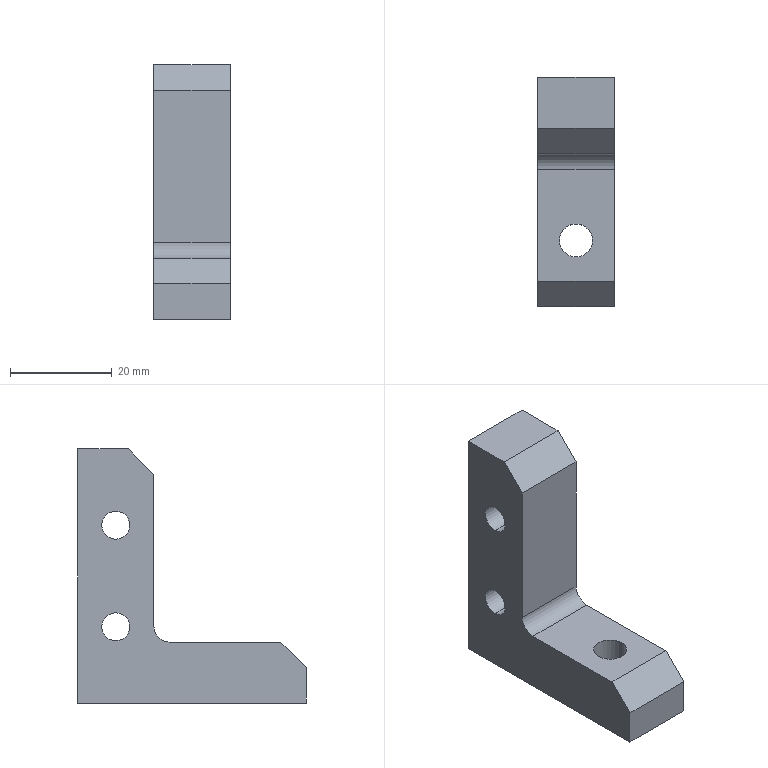Part | SolidWorks | features HoleWzd 2, Chamfer 1, Extrusion 1, Fillet 1, ICE 1 | 1 solid | 17 faces | box 15 x 45 x 50 mm | volume 15193 mm3 | plane 10 | cylinder 7 | commonest cylinder face diameters 5.5 x4 6.5 x2 6 x1
STEP:
#1=CARTESIAN_POINT('',(-7.5,0.,-7.25));
#2=VERTEX_POINT('',#1);
#3=CARTESIAN_POINT('',(-7.5,0.,-12.75));
#4=VERTEX_POINT('',#3);
#5=CARTESIAN_POINT('',(-7.5,0.,-10.));
#6=DIRECTION('',(1.,0.,0.));
#7=DIRECTION('',(0.,0.,-1.));
#8=AXIS2_PLACEMENT_3D('',#5,#6,#7);
#9=CIRCLE('',#8,2.75);
#10=EDGE_CURVE('',#2,#4,#9,.T.);
#11=ORIENTED_EDGE('',*,*,#10,.F.);
#12=CARTESIAN_POINT('',(7.5,0.,-7.25));
#13=VERTEX_POINT('',#12);
#14=CARTESIAN_POINT('',(7.5,0.,-7.25));
#15=DIRECTION('',(1.,0.,0.));
#16=VECTOR('',#15,1000.);
#17=LINE('',#14,#16);
#18=EDGE_CURVE('',#2,#13,#17,.T.);
#19=ORIENTED_EDGE('',*,*,#18,.T.);
#20=CARTESIAN_POINT('',(7.5,0.,-12.75));
#21=VERTEX_POINT('',#20);
#22=CARTESIAN_POINT('',(7.5,0.,-10.));
#23=DIRECTION('',(1.,0.,0.));
#24=DIRECTION('',(0.,0.,-1.));
#25=AXIS2_PLACEMENT_3D('',#22,#23,#24);
#26=CIRCLE('',#25,2.75);
#27=EDGE_CURVE('',#13,#21,#26,.T.);
#28=ORIENTED_EDGE('',*,*,#27,.T.);
#29=CARTESIAN_POINT('',(7.5,0.,-12.75));
#30=DIRECTION('',(1.,0.,0.));
#31=VECTOR('',#30,1000.);
#32=LINE('',#29,#31);
#33=EDGE_CURVE('',#4,#21,#32,.T.);
#34=ORIENTED_EDGE('',*,*,#33,.F.);
#35=EDGE_LOOP('',(#11,#19,#28,#34));
#36=FACE_OUTER_BOUND('',#35,.T.);
#37=CARTESIAN_POINT('',(7.5,0.,-10.));
#38=DIRECTION('',(1.,0.,0.));
#39=DIRECTION('',(0.,0.,-1.));
#40=AXIS2_PLACEMENT_3D('',#37,#38,#39);
#41=CYLINDRICAL_SURFACE('',#40,2.75);
#42=ADVANCED_FACE('',(#36),#41,.F.);
#43=CARTESIAN_POINT('',(-7.5,0.,12.75));
#44=VERTEX_POINT('',#43);
#45=CARTESIAN_POINT('',(-7.5,0.,7.25));
#46=VERTEX_POINT('',#45);
#47=CARTESIAN_POINT('',(-7.5,0.,10.));
#48=DIRECTION('',(1.,0.,0.));
#49=DIRECTION('',(0.,0.,-1.));
#50=AXIS2_PLACEMENT_3D('',#47,#48,#49);
#51=CIRCLE('',#50,2.75);
#52=EDGE_CURVE('',#44,#46,#51,.T.);
#53=ORIENTED_EDGE('',*,*,#52,.F.);
#54=CARTESIAN_POINT('',(7.5,0.,12.75));
#55=VERTEX_POINT('',#54);
#56=CARTESIAN_POINT('',(7.5,0.,12.75));
#57=DIRECTION('',(1.,0.,0.));
#58=VECTOR('',#57,1000.);
#59=LINE('',#56,#58);
#60=EDGE_CURVE('',#44,#55,#59,.T.);
#61=ORIENTED_EDGE('',*,*,#60,.T.);
#62=CARTESIAN_POINT('',(7.5,0.,7.25));
#63=VERTEX_POINT('',#62);
#64=CARTESIAN_POINT('',(7.5,0.,10.));
#65=DIRECTION('',(1.,0.,0.));
#66=DIRECTION('',(0.,0.,-1.));
#67=AXIS2_PLACEMENT_3D('',#64,#65,#66);
#68=CIRCLE('',#67,2.75);
#69=EDGE_CURVE('',#55,#63,#68,.T.);
#70=ORIENTED_EDGE('',*,*,#69,.T.);
#71=CARTESIAN_POINT('',(7.5,0.,7.25));
#72=DIRECTION('',(1.,0.,0.));
#73=VECTOR('',#72,1000.);
#74=LINE('',#71,#73);
#75=EDGE_CURVE('',#46,#63,#74,.T.);
#76=ORIENTED_EDGE('',*,*,#75,.F.);
#77=EDGE_LOOP('',(#53,#61,#70,#76));
#78=FACE_OUTER_BOUND('',#77,.T.);
#79=CARTESIAN_POINT('',(7.5,0.,10.));
#80=DIRECTION('',(1.,0.,0.));
#81=DIRECTION('',(0.,0.,-1.));
#82=AXIS2_PLACEMENT_3D('',#79,#80,#81);
#83=CYLINDRICAL_SURFACE('',#82,2.75);
#84=ADVANCED_FACE('',(#78),#83,.F.);
#85=CARTESIAN_POINT('',(-3.25,-24.5,-25.));
#86=VERTEX_POINT('',#85);
#87=CARTESIAN_POINT('',(3.25,-24.5,-25.));
#88=VERTEX_POINT('',#87);
#89=CARTESIAN_POINT('',(0.,-24.5,-25.));
#90=DIRECTION('',(0.,0.,1.));
#91=DIRECTION('',(1.,0.,0.));
#92=AXIS2_PLACEMENT_3D('',#89,#90,#91);
#93=CIRCLE('',#92,3.25);
#94=EDGE_CURVE('',#86,#88,#93,.T.);
#95=ORIENTED_EDGE('',*,*,#94,.F.);
#96=CARTESIAN_POINT('',(-3.25,-24.5,-13.));
#97=VERTEX_POINT('',#96);
#98=CARTESIAN_POINT('',(-3.25,-24.5,-13.));
#99=DIRECTION('',(0.,0.,1.));
#100=VECTOR('',#99,1000.);
#101=LINE('',#98,#100);
#102=EDGE_CURVE('',#86,#97,#101,.T.);
#103=ORIENTED_EDGE('',*,*,#102,.T.);
#104=CARTESIAN_POINT('',(3.25,-24.5,-13.));
#105=VERTEX_POINT('',#104);
#106=CARTESIAN_POINT('',(0.,-24.5,-13.));
#107=DIRECTION('',(0.,0.,1.));
#108=DIRECTION('',(1.,0.,0.));
#109=AXIS2_PLACEMENT_3D('',#106,#107,#108);
#110=CIRCLE('',#109,3.25);
#111=EDGE_CURVE('',#97,#105,#110,.T.);
#112=ORIENTED_EDGE('',*,*,#111,.T.);
#113=CARTESIAN_POINT('',(3.25,-24.5,-13.));
#114=DIRECTION('',(0.,0.,1.));
#115=VECTOR('',#114,1000.);
#116=LINE('',#113,#115);
#117=EDGE_CURVE('',#88,#105,#116,.T.);
#118=ORIENTED_EDGE('',*,*,#117,.F.);
#119=EDGE_LOOP('',(#95,#103,#112,#118));
#120=FACE_OUTER_BOUND('',#119,.T.);
#121=CARTESIAN_POINT('',(0.,-24.5,-13.));
#122=DIRECTION('',(0.,0.,1.));
#123=DIRECTION('',(1.,0.,0.));
#124=AXIS2_PLACEMENT_3D('',#121,#122,#123);
#125=CYLINDRICAL_SURFACE('',#124,3.25);
#126=ADVANCED_FACE('',(#120),#125,.F.);
#127=CARTESIAN_POINT('',(7.5,0.,-10.));
#128=DIRECTION('',(1.,0.,0.));
#129=DIRECTION('',(0.,0.,-1.));
#130=AXIS2_PLACEMENT_3D('',#127,#128,#129);
#131=CIRCLE('',#130,2.75);
#132=EDGE_CURVE('',#21,#13,#131,.T.);
#133=ORIENTED_EDGE('',*,*,#132,.F.);
#134=ORIENTED_EDGE('',*,*,#27,.F.);
#135=EDGE_LOOP('',(#133,#134));
#136=FACE_BOUND('',#135,.T.);
#137=CARTESIAN_POINT('',(7.5,0.,10.));
#138=DIRECTION('',(1.,0.,0.));
#139=DIRECTION('',(0.,0.,-1.));
#140=AXIS2_PLACEMENT_3D('',#137,#138,#139);
#141=CIRCLE('',#140,2.75);
#142=EDGE_CURVE('',#63,#55,#141,.T.);
#143=ORIENTED_EDGE('',*,*,#142,.F.);
#144=ORIENTED_EDGE('',*,*,#69,.F.);
#145=EDGE_LOOP('',(#143,#144));
#146=FACE_BOUND('',#145,.T.);
#147=CARTESIAN_POINT('',(7.5,-2.5,25.));
#148=VERTEX_POINT('',#147);
#149=CARTESIAN_POINT('',(7.5,7.5,25.));
#150=VERTEX_POINT('',#149);
#151=CARTESIAN_POINT('',(7.5,-7.5,25.));
#152=DIRECTION('',(0.,1.,0.));
#153=VECTOR('',#152,1000.);
#154=LINE('',#151,#153);
#155=EDGE_CURVE('',#148,#150,#154,.T.);
#156=ORIENTED_EDGE('',*,*,#155,.F.);
#157=CARTESIAN_POINT('',(7.5,-7.5,20.));
#158=VERTEX_POINT('',#157);
#159=CARTESIAN_POINT('',(7.5,-2.5,25.));
#160=DIRECTION('',(0.,-0.7071,-0.7071));
#161=VECTOR('',#160,1000.);
#162=LINE('',#159,#161);
#163=EDGE_CURVE('',#148,#158,#162,.T.);
#164=ORIENTED_EDGE('',*,*,#163,.T.);
#165=CARTESIAN_POINT('',(7.5,-7.5,-10.));
#166=VERTEX_POINT('',#165);
#167=CARTESIAN_POINT('',(7.5,-7.5,25.));
#168=DIRECTION('',(0.,0.,-1.));
#169=VECTOR('',#168,1000.);
#170=LINE('',#167,#169);
#171=EDGE_CURVE('',#158,#166,#170,.T.);
#172=ORIENTED_EDGE('',*,*,#171,.T.);
#173=CARTESIAN_POINT('',(7.5,-10.5,-13.));
#174=VERTEX_POINT('',#173);
#175=CARTESIAN_POINT('',(7.5,-10.5,-10.));
#176=DIRECTION('',(-1.,0.,0.));
#177=DIRECTION('',(0.,0.,1.));
#178=AXIS2_PLACEMENT_3D('',#175,#176,#177);
#179=CIRCLE('',#178,3.);
#180=EDGE_CURVE('',#166,#174,#179,.T.);
#181=ORIENTED_EDGE('',*,*,#180,.T.);
#182=CARTESIAN_POINT('',(7.5,-32.5,-13.));
#183=VERTEX_POINT('',#182);
#184=CARTESIAN_POINT('',(7.5,-7.5,-13.));
#185=DIRECTION('',(0.,-1.,0.));
#186=VECTOR('',#185,1000.);
#187=LINE('',#184,#186);
#188=EDGE_CURVE('',#174,#183,#187,.T.);
#189=ORIENTED_EDGE('',*,*,#188,.T.);
#190=CARTESIAN_POINT('',(7.5,-37.5,-18.));
#191=VERTEX_POINT('',#190);
#192=CARTESIAN_POINT('',(7.5,-37.5,-18.));
#193=DIRECTION('',(0.,-0.7071,-0.7071));
#194=VECTOR('',#193,1000.);
#195=LINE('',#192,#194);
#196=EDGE_CURVE('',#183,#191,#195,.T.);
#197=ORIENTED_EDGE('',*,*,#196,.T.);
#198=CARTESIAN_POINT('',(7.5,-37.5,-25.));
#199=VERTEX_POINT('',#198);
#200=CARTESIAN_POINT('',(7.5,-37.5,-13.));
#201=DIRECTION('',(0.,0.,-1.));
#202=VECTOR('',#201,1000.);
#203=LINE('',#200,#202);
#204=EDGE_CURVE('',#191,#199,#203,.T.);
#205=ORIENTED_EDGE('',*,*,#204,.T.);
#206=CARTESIAN_POINT('',(7.5,7.5,-25.));
#207=VERTEX_POINT('',#206);
#208=CARTESIAN_POINT('',(7.5,-7.5,-25.));
#209=DIRECTION('',(0.,1.,0.));
#210=VECTOR('',#209,1000.);
#211=LINE('',#208,#210);
#212=EDGE_CURVE('',#199,#207,#211,.T.);
#213=ORIENTED_EDGE('',*,*,#212,.T.);
#214=CARTESIAN_POINT('',(7.5,7.5,25.));
#215=DIRECTION('',(0.,0.,-1.));
#216=VECTOR('',#215,1000.);
#217=LINE('',#214,#216);
#218=EDGE_CURVE('',#150,#207,#217,.T.);
#219=ORIENTED_EDGE('',*,*,#218,.F.);
#220=EDGE_LOOP('',(#156,#164,#172,#181,#189,#197,#205,#213,#219));
#221=FACE_OUTER_BOUND('',#220,.T.);
#222=CARTESIAN_POINT('',(7.5,-7.5,25.));
#223=DIRECTION('',(-1.,0.,0.));
#224=DIRECTION('',(0.,0.,1.));
#225=AXIS2_PLACEMENT_3D('',#222,#223,#224);
#226=PLANE('',#225);
#227=ADVANCED_FACE('',(#136,#146,#221),#226,.F.);
#228=CARTESIAN_POINT('',(-7.5,7.5,-25.));
#229=VERTEX_POINT('',#228);
#230=CARTESIAN_POINT('',(-7.5,7.5,-25.));
#231=DIRECTION('',(-1.,0.,0.));
#232=VECTOR('',#231,1000.);
#233=LINE('',#230,#232);
#234=EDGE_CURVE('',#207,#229,#233,.T.);
#235=ORIENTED_EDGE('',*,*,#234,.T.);
#236=CARTESIAN_POINT('',(-7.5,7.5,25.));
#237=VERTEX_POINT('',#236);
#238=CARTESIAN_POINT('',(-7.5,7.5,25.));
#239=DIRECTION('',(0.,0.,-1.));
#240=VECTOR('',#239,1000.);
#241=LINE('',#238,#240);
#242=EDGE_CURVE('',#237,#229,#241,.T.);
#243=ORIENTED_EDGE('',*,*,#242,.F.);
#244=CARTESIAN_POINT('',(-7.5,7.5,25.));
#245=DIRECTION('',(-1.,0.,0.));
#246=VECTOR('',#245,1000.);
#247=LINE('',#244,#246);
#248=EDGE_CURVE('',#150,#237,#247,.T.);
#249=ORIENTED_EDGE('',*,*,#248,.F.);
#250=ORIENTED_EDGE('',*,*,#218,.T.);
#251=EDGE_LOOP('',(#235,#243,#249,#250));
#252=FACE_OUTER_BOUND('',#251,.T.);
#253=CARTESIAN_POINT('',(-7.5,7.5,25.));
#254=DIRECTION('',(0.,-1.,0.));
#255=DIRECTION('',(0.,0.,-1.));
#256=AXIS2_PLACEMENT_3D('',#253,#254,#255);
#257=PLANE('',#256);
#258=ADVANCED_FACE('',(#252),#257,.F.);
#259=CARTESIAN_POINT('',(-7.5,0.,-10.));
#260=DIRECTION('',(1.,0.,0.));
#261=DIRECTION('',(0.,0.,-1.));
#262=AXIS2_PLACEMENT_3D('',#259,#260,#261);
#263=CIRCLE('',#262,2.75);
#264=EDGE_CURVE('',#4,#2,#263,.T.);
#265=ORIENTED_EDGE('',*,*,#264,.T.);
#266=ORIENTED_EDGE('',*,*,#10,.T.);
#267=EDGE_LOOP('',(#265,#266));
#268=FACE_BOUND('',#267,.T.);
#269=CARTESIAN_POINT('',(-7.5,0.,10.));
#270=DIRECTION('',(1.,0.,0.));
#271=DIRECTION('',(0.,0.,-1.));
#272=AXIS2_PLACEMENT_3D('',#269,#270,#271);
#273=CIRCLE('',#272,2.75);
#274=EDGE_CURVE('',#46,#44,#273,.T.);
#275=ORIENTED_EDGE('',*,*,#274,.T.);
#276=ORIENTED_EDGE('',*,*,#52,.T.);
#277=EDGE_LOOP('',(#275,#276));
#278=FACE_BOUND('',#277,.T.);
#279=CARTESIAN_POINT('',(-7.5,-7.5,20.));
#280=VERTEX_POINT('',#279);
#281=CARTESIAN_POINT('',(-7.5,-7.5,-10.));
#282=VERTEX_POINT('',#281);
#283=CARTESIAN_POINT('',(-7.5,-7.5,25.));
#284=DIRECTION('',(0.,0.,-1.));
#285=VECTOR('',#284,1000.);
#286=LINE('',#283,#285);
#287=EDGE_CURVE('',#280,#282,#286,.T.);
#288=ORIENTED_EDGE('',*,*,#287,.F.);
#289=CARTESIAN_POINT('',(-7.5,-2.5,25.));
#290=VERTEX_POINT('',#289);
#291=CARTESIAN_POINT('',(-7.5,-2.5,25.));
#292=DIRECTION('',(0.,0.7071,0.7071));
#293=VECTOR('',#292,1000.);
#294=LINE('',#291,#293);
#295=EDGE_CURVE('',#280,#290,#294,.T.);
#296=ORIENTED_EDGE('',*,*,#295,.T.);
#297=CARTESIAN_POINT('',(-7.5,-7.5,25.));
#298=DIRECTION('',(0.,-1.,0.));
#299=VECTOR('',#298,1000.);
#300=LINE('',#297,#299);
#301=EDGE_CURVE('',#237,#290,#300,.T.);
#302=ORIENTED_EDGE('',*,*,#301,.F.);
#303=ORIENTED_EDGE('',*,*,#242,.T.);
#304=CARTESIAN_POINT('',(-7.5,-37.5,-25.));
#305=VERTEX_POINT('',#304);
#306=CARTESIAN_POINT('',(-7.5,-7.5,-25.));
#307=DIRECTION('',(0.,-1.,0.));
#308=VECTOR('',#307,1000.);
#309=LINE('',#306,#308);
#310=EDGE_CURVE('',#229,#305,#309,.T.);
#311=ORIENTED_EDGE('',*,*,#310,.T.);
#312=CARTESIAN_POINT('',(-7.5,-37.5,-18.));
#313=VERTEX_POINT('',#312);
#314=CARTESIAN_POINT('',(-7.5,-37.5,-13.));
#315=DIRECTION('',(0.,0.,-1.));
#316=VECTOR('',#315,1000.);
#317=LINE('',#314,#316);
#318=EDGE_CURVE('',#313,#305,#317,.T.);
#319=ORIENTED_EDGE('',*,*,#318,.F.);
#320=CARTESIAN_POINT('',(-7.5,-32.5,-13.));
#321=VERTEX_POINT('',#320);
#322=CARTESIAN_POINT('',(-7.5,-37.5,-18.));
#323=DIRECTION('',(0.,0.7071,0.7071));
#324=VECTOR('',#323,1000.);
#325=LINE('',#322,#324);
#326=EDGE_CURVE('',#313,#321,#325,.T.);
#327=ORIENTED_EDGE('',*,*,#326,.T.);
#328=CARTESIAN_POINT('',(-7.5,-10.5,-13.));
#329=VERTEX_POINT('',#328);
#330=CARTESIAN_POINT('',(-7.5,-7.5,-13.));
#331=DIRECTION('',(0.,1.,0.));
#332=VECTOR('',#331,1000.);
#333=LINE('',#330,#332);
#334=EDGE_CURVE('',#321,#329,#333,.T.);
#335=ORIENTED_EDGE('',*,*,#334,.T.);
#336=CARTESIAN_POINT('',(-7.5,-10.5,-10.));
#337=DIRECTION('',(1.,0.,0.));
#338=DIRECTION('',(0.,0.,-1.));
#339=AXIS2_PLACEMENT_3D('',#336,#337,#338);
#340=CIRCLE('',#339,3.);
#341=EDGE_CURVE('',#329,#282,#340,.T.);
#342=ORIENTED_EDGE('',*,*,#341,.T.);
#343=EDGE_LOOP('',(#288,#296,#302,#303,#311,#319,#327,#335,#342));
#344=FACE_OUTER_BOUND('',#343,.T.);
#345=CARTESIAN_POINT('',(-7.5,-7.5,25.));
#346=DIRECTION('',(1.,0.,0.));
#347=DIRECTION('',(0.,0.,-1.));
#348=AXIS2_PLACEMENT_3D('',#345,#346,#347);
#349=PLANE('',#348);
#350=ADVANCED_FACE('',(#268,#278,#344),#349,.F.);
#351=ORIENTED_EDGE('',*,*,#171,.F.);
#352=CARTESIAN_POINT('',(-7.5,-7.5,20.));
#353=DIRECTION('',(-1.,0.,0.));
#354=VECTOR('',#353,1000.);
#355=LINE('',#352,#354);
#356=EDGE_CURVE('',#158,#280,#355,.T.);
#357=ORIENTED_EDGE('',*,*,#356,.T.);
#358=ORIENTED_EDGE('',*,*,#287,.T.);
#359=CARTESIAN_POINT('',(-7.5,-7.5,-10.));
#360=DIRECTION('',(1.,0.,0.));
#361=VECTOR('',#360,1000.);
#362=LINE('',#359,#361);
#363=EDGE_CURVE('',#282,#166,#362,.T.);
#364=ORIENTED_EDGE('',*,*,#363,.T.);
#365=EDGE_LOOP('',(#351,#357,#358,#364));
#366=FACE_OUTER_BOUND('',#365,.T.);
#367=CARTESIAN_POINT('',(-7.5,-7.5,25.));
#368=DIRECTION('',(0.,1.,0.));
#369=DIRECTION('',(0.,0.,1.));
#370=AXIS2_PLACEMENT_3D('',#367,#368,#369);
#371=PLANE('',#370);
#372=ADVANCED_FACE('',(#366),#371,.F.);
#373=ORIENTED_EDGE('',*,*,#301,.T.);
#374=CARTESIAN_POINT('',(0.,-2.5,25.));
#375=DIRECTION('',(1.,0.,0.));
#376=VECTOR('',#375,1000.);
#377=LINE('',#374,#376);
#378=EDGE_CURVE('',#290,#148,#377,.T.);
#379=ORIENTED_EDGE('',*,*,#378,.T.);
#380=ORIENTED_EDGE('',*,*,#155,.T.);
#381=ORIENTED_EDGE('',*,*,#248,.T.);
#382=EDGE_LOOP('',(#373,#379,#380,#381));
#383=FACE_OUTER_BOUND('',#382,.T.);
#384=CARTESIAN_POINT('',(0.,0.,25.));
#385=DIRECTION('',(0.,0.,-1.));
#386=DIRECTION('',(-1.,0.,0.));
#387=AXIS2_PLACEMENT_3D('',#384,#385,#386);
#388=PLANE('',#387);
#389=ADVANCED_FACE('',(#383),#388,.F.);
#390=CARTESIAN_POINT('',(0.,-24.5,-25.));
#391=DIRECTION('',(0.,0.,1.));
#392=DIRECTION('',(1.,0.,0.));
#393=AXIS2_PLACEMENT_3D('',#390,#391,#392);
#394=CIRCLE('',#393,3.25);
#395=EDGE_CURVE('',#88,#86,#394,.T.);
#396=ORIENTED_EDGE('',*,*,#395,.T.);
#397=ORIENTED_EDGE('',*,*,#94,.T.);
#398=EDGE_LOOP('',(#396,#397));
#399=FACE_BOUND('',#398,.T.);
#400=ORIENTED_EDGE('',*,*,#212,.F.);
#401=CARTESIAN_POINT('',(-7.5,-37.5,-25.));
#402=DIRECTION('',(-1.,0.,0.));
#403=VECTOR('',#402,1000.);
#404=LINE('',#401,#403);
#405=EDGE_CURVE('',#199,#305,#404,.T.);
#406=ORIENTED_EDGE('',*,*,#405,.T.);
#407=ORIENTED_EDGE('',*,*,#310,.F.);
#408=ORIENTED_EDGE('',*,*,#234,.F.);
#409=EDGE_LOOP('',(#400,#406,#407,#408));
#410=FACE_OUTER_BOUND('',#409,.T.);
#411=CARTESIAN_POINT('',(0.,0.,-25.));
#412=DIRECTION('',(0.,0.,-1.));
#413=DIRECTION('',(-1.,0.,0.));
#414=AXIS2_PLACEMENT_3D('',#411,#412,#413);
#415=PLANE('',#414);
#416=ADVANCED_FACE('',(#399,#410),#415,.T.);
#417=ORIENTED_EDGE('',*,*,#204,.F.);
#418=CARTESIAN_POINT('',(-7.5,-37.5,-18.));
#419=DIRECTION('',(-1.,0.,0.));
#420=VECTOR('',#419,1000.);
#421=LINE('',#418,#420);
#422=EDGE_CURVE('',#191,#313,#421,.T.);
#423=ORIENTED_EDGE('',*,*,#422,.T.);
#424=ORIENTED_EDGE('',*,*,#318,.T.);
#425=ORIENTED_EDGE('',*,*,#405,.F.);
#426=EDGE_LOOP('',(#417,#423,#424,#425));
#427=FACE_OUTER_BOUND('',#426,.T.);
#428=CARTESIAN_POINT('',(-7.5,-37.5,-13.));
#429=DIRECTION('',(0.,-1.,0.));
#430=DIRECTION('',(1.,0.,0.));
#431=AXIS2_PLACEMENT_3D('',#428,#429,#430);
#432=PLANE('',#431);
#433=ADVANCED_FACE('',(#427),#432,.T.);
#434=CARTESIAN_POINT('',(0.,-24.5,-13.));
#435=DIRECTION('',(0.,0.,1.));
#436=DIRECTION('',(1.,0.,0.));
#437=AXIS2_PLACEMENT_3D('',#434,#435,#436);
#438=CIRCLE('',#437,3.25);
#439=EDGE_CURVE('',#105,#97,#438,.T.);
#440=ORIENTED_EDGE('',*,*,#439,.F.);
#441=ORIENTED_EDGE('',*,*,#111,.F.);
#442=EDGE_LOOP('',(#440,#441));
#443=FACE_BOUND('',#442,.T.);
#444=ORIENTED_EDGE('',*,*,#334,.F.);
#445=CARTESIAN_POINT('',(0.,-32.5,-13.));
#446=DIRECTION('',(1.,0.,0.));
#447=VECTOR('',#446,1000.);
#448=LINE('',#445,#447);
#449=EDGE_CURVE('',#321,#183,#448,.T.);
#450=ORIENTED_EDGE('',*,*,#449,.T.);
#451=ORIENTED_EDGE('',*,*,#188,.F.);
#452=CARTESIAN_POINT('',(0.,-10.5,-13.));
#453=DIRECTION('',(-1.,0.,0.));
#454=VECTOR('',#453,1000.);
#455=LINE('',#452,#454);
#456=EDGE_CURVE('',#174,#329,#455,.T.);
#457=ORIENTED_EDGE('',*,*,#456,.T.);
#458=EDGE_LOOP('',(#444,#450,#451,#457));
#459=FACE_OUTER_BOUND('',#458,.T.);
#460=CARTESIAN_POINT('',(0.,0.,-13.));
#461=DIRECTION('',(0.,0.,1.));
#462=DIRECTION('',(1.,0.,0.));
#463=AXIS2_PLACEMENT_3D('',#460,#461,#462);
#464=PLANE('',#463);
#465=ADVANCED_FACE('',(#443,#459),#464,.T.);
#466=ORIENTED_EDGE('',*,*,#102,.F.);
#467=ORIENTED_EDGE('',*,*,#395,.F.);
#468=ORIENTED_EDGE('',*,*,#117,.T.);
#469=ORIENTED_EDGE('',*,*,#439,.T.);
#470=EDGE_LOOP('',(#466,#467,#468,#469));
#471=FACE_OUTER_BOUND('',#470,.T.);
#472=CARTESIAN_POINT('',(0.,-24.5,-13.));
#473=DIRECTION('',(0.,0.,1.));
#474=DIRECTION('',(1.,0.,0.));
#475=AXIS2_PLACEMENT_3D('',#472,#473,#474);
#476=CYLINDRICAL_SURFACE('',#475,3.25);
#477=ADVANCED_FACE('',(#471),#476,.F.);
#478=ORIENTED_EDGE('',*,*,#341,.F.);
#479=ORIENTED_EDGE('',*,*,#456,.F.);
#480=ORIENTED_EDGE('',*,*,#180,.F.);
#481=ORIENTED_EDGE('',*,*,#363,.F.);
#482=EDGE_LOOP('',(#478,#479,#480,#481));
#483=FACE_OUTER_BOUND('',#482,.T.);
#484=CARTESIAN_POINT('',(-7.5,-10.5,-10.));
#485=DIRECTION('',(1.,0.,0.));
#486=DIRECTION('',(0.,0.,-1.));
#487=AXIS2_PLACEMENT_3D('',#484,#485,#486);
#488=CYLINDRICAL_SURFACE('',#487,3.);
#489=ADVANCED_FACE('',(#483),#488,.F.);
#490=ORIENTED_EDGE('',*,*,#295,.F.);
#491=ORIENTED_EDGE('',*,*,#356,.F.);
#492=ORIENTED_EDGE('',*,*,#163,.F.);
#493=ORIENTED_EDGE('',*,*,#378,.F.);
#494=EDGE_LOOP('',(#490,#491,#492,#493));
#495=FACE_OUTER_BOUND('',#494,.T.);
#496=CARTESIAN_POINT('',(0.,-2.5,25.));
#497=DIRECTION('',(0.,0.7071,-0.7071));
#498=DIRECTION('',(1.,0.,0.));
#499=AXIS2_PLACEMENT_3D('',#496,#497,#498);
#500=PLANE('',#499);
#501=ADVANCED_FACE('',(#495),#500,.F.);
#502=ORIENTED_EDGE('',*,*,#196,.F.);
#503=ORIENTED_EDGE('',*,*,#449,.F.);
#504=ORIENTED_EDGE('',*,*,#326,.F.);
#505=ORIENTED_EDGE('',*,*,#422,.F.);
#506=EDGE_LOOP('',(#502,#503,#504,#505));
#507=FACE_OUTER_BOUND('',#506,.T.);
#508=CARTESIAN_POINT('',(-7.5,-37.5,-18.));
#509=DIRECTION('',(0.,0.7071,-0.7071));
#510=DIRECTION('',(-1.,0.,0.));
#511=AXIS2_PLACEMENT_3D('',#508,#509,#510);
#512=PLANE('',#511);
#513=ADVANCED_FACE('',(#507),#512,.F.);
#514=ORIENTED_EDGE('',*,*,#60,.F.);
#515=ORIENTED_EDGE('',*,*,#274,.F.);
#516=ORIENTED_EDGE('',*,*,#75,.T.);
#517=ORIENTED_EDGE('',*,*,#142,.T.);
#518=EDGE_LOOP('',(#514,#515,#516,#517));
#519=FACE_OUTER_BOUND('',#518,.T.);
#520=CARTESIAN_POINT('',(7.5,0.,10.));
#521=DIRECTION('',(1.,0.,0.));
#522=DIRECTION('',(0.,0.,-1.));
#523=AXIS2_PLACEMENT_3D('',#520,#521,#522);
#524=CYLINDRICAL_SURFACE('',#523,2.75);
#525=ADVANCED_FACE('',(#519),#524,.F.);
#526=ORIENTED_EDGE('',*,*,#18,.F.);
#527=ORIENTED_EDGE('',*,*,#264,.F.);
#528=ORIENTED_EDGE('',*,*,#33,.T.);
#529=ORIENTED_EDGE('',*,*,#132,.T.);
#530=EDGE_LOOP('',(#526,#527,#528,#529));
#531=FACE_OUTER_BOUND('',#530,.T.);
#532=CARTESIAN_POINT('',(7.5,0.,-10.));
#533=DIRECTION('',(1.,0.,0.));
#534=DIRECTION('',(0.,0.,-1.));
#535=AXIS2_PLACEMENT_3D('',#532,#533,#534);
#536=CYLINDRICAL_SURFACE('',#535,2.75);
#537=ADVANCED_FACE('',(#531),#536,.F.);
#538=CLOSED_SHELL('',(#42,#84,#126,#227,#258,#350,#372,#389,#416,#433,#465,#477,#489,#501,#513,#525,#537));
#539=MANIFOLD_SOLID_BREP('',#538);
#540=CARTESIAN_POINT('',(0.,0.,0.));
#541=DIRECTION('',(0.,0.,1.));
#542=DIRECTION('',(1.,0.,0.));
#543=AXIS2_PLACEMENT_3D('',#540,#541,#542);
#544=(LENGTH_UNIT()NAMED_UNIT(*)SI_UNIT(.MILLI.,.METRE.));
#545=UNCERTAINTY_MEASURE_WITH_UNIT(LENGTH_MEASURE(0.00001),#544,'','');
#546=(NAMED_UNIT(*)PLANE_ANGLE_UNIT()SI_UNIT($,.RADIAN.));
#547=(NAMED_UNIT(*)SI_UNIT($,.STERADIAN.)SOLID_ANGLE_UNIT());
#548=(GEOMETRIC_REPRESENTATION_CONTEXT(3)GLOBAL_UNCERTAINTY_ASSIGNED_CONTEXT((#545))GLOBAL_UNIT_ASSIGNED_CONTEXT((#544,#546,#547))REPRESENTATION_CONTEXT('',''));
#549=ADVANCED_BREP_SHAPE_REPRESENTATION('',(#539,#543),#548);